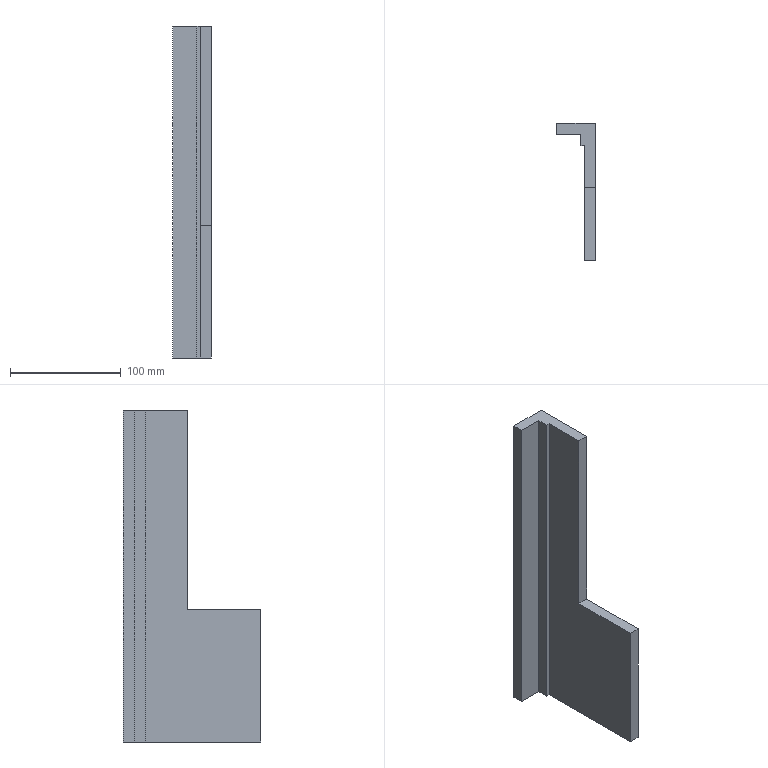Part | STEP file | Platform 2 slider plate 2 | 1 solid | 12 faces | box 35 x 124 x 300 mm | volume 337200 mm3 | plane 12
STEP:
#1=CARTESIAN_POINT('',(0.,0.,-150.));
#2=VERTEX_POINT('',#1);
#3=CARTESIAN_POINT('',(0.,-10.,-150.));
#4=VERTEX_POINT('',#3);
#5=CARTESIAN_POINT('',(0.,-10.,-150.));
#6=DIRECTION('',(0.,-1.,0.));
#7=VECTOR('',#6,1000.);
#8=LINE('',#5,#7);
#9=EDGE_CURVE('',#2,#4,#8,.T.);
#10=ORIENTED_EDGE('',*,*,#9,.T.);
#11=CARTESIAN_POINT('',(0.,-10.,150.));
#12=VERTEX_POINT('',#11);
#13=CARTESIAN_POINT('',(0.,-10.,150.));
#14=DIRECTION('',(0.,0.,-1.));
#15=VECTOR('',#14,1000.);
#16=LINE('',#13,#15);
#17=EDGE_CURVE('',#12,#4,#16,.T.);
#18=ORIENTED_EDGE('',*,*,#17,.F.);
#19=CARTESIAN_POINT('',(0.,0.,150.));
#20=VERTEX_POINT('',#19);
#21=CARTESIAN_POINT('',(0.,-10.,150.));
#22=DIRECTION('',(0.,-1.,0.));
#23=VECTOR('',#22,1000.);
#24=LINE('',#21,#23);
#25=EDGE_CURVE('',#20,#12,#24,.T.);
#26=ORIENTED_EDGE('',*,*,#25,.F.);
#27=CARTESIAN_POINT('',(0.,0.,150.));
#28=DIRECTION('',(0.,0.,-1.));
#29=VECTOR('',#28,1000.);
#30=LINE('',#27,#29);
#31=EDGE_CURVE('',#20,#2,#30,.T.);
#32=ORIENTED_EDGE('',*,*,#31,.T.);
#33=EDGE_LOOP('',(#10,#18,#26,#32));
#34=FACE_OUTER_BOUND('',#33,.T.);
#35=CARTESIAN_POINT('',(0.,-10.,150.));
#36=DIRECTION('',(1.,0.,0.));
#37=DIRECTION('',(0.,0.,-1.));
#38=AXIS2_PLACEMENT_3D('',#35,#36,#37);
#39=PLANE('',#38);
#40=ADVANCED_FACE('',(#34),#39,.F.);
#41=CARTESIAN_POINT('',(22.,-10.,-150.));
#42=VERTEX_POINT('',#41);
#43=CARTESIAN_POINT('',(22.,-10.,-150.));
#44=DIRECTION('',(1.,0.,0.));
#45=VECTOR('',#44,1000.);
#46=LINE('',#43,#45);
#47=EDGE_CURVE('',#4,#42,#46,.T.);
#48=ORIENTED_EDGE('',*,*,#47,.T.);
#49=CARTESIAN_POINT('',(22.,-10.,150.));
#50=VERTEX_POINT('',#49);
#51=CARTESIAN_POINT('',(22.,-10.,150.));
#52=DIRECTION('',(0.,0.,-1.));
#53=VECTOR('',#52,1000.);
#54=LINE('',#51,#53);
#55=EDGE_CURVE('',#50,#42,#54,.T.);
#56=ORIENTED_EDGE('',*,*,#55,.F.);
#57=CARTESIAN_POINT('',(22.,-10.,150.));
#58=DIRECTION('',(1.,0.,0.));
#59=VECTOR('',#58,1000.);
#60=LINE('',#57,#59);
#61=EDGE_CURVE('',#12,#50,#60,.T.);
#62=ORIENTED_EDGE('',*,*,#61,.F.);
#63=ORIENTED_EDGE('',*,*,#17,.T.);
#64=EDGE_LOOP('',(#48,#56,#62,#63));
#65=FACE_OUTER_BOUND('',#64,.T.);
#66=CARTESIAN_POINT('',(22.,-10.,150.));
#67=DIRECTION('',(0.,1.,0.));
#68=DIRECTION('',(-1.,0.,0.));
#69=AXIS2_PLACEMENT_3D('',#66,#67,#68);
#70=PLANE('',#69);
#71=ADVANCED_FACE('',(#65),#70,.F.);
#72=CARTESIAN_POINT('',(22.,-20.,-150.));
#73=VERTEX_POINT('',#72);
#74=CARTESIAN_POINT('',(22.,-124.,-150.));
#75=DIRECTION('',(0.,-1.,0.));
#76=VECTOR('',#75,1000.);
#77=LINE('',#74,#76);
#78=EDGE_CURVE('',#42,#73,#77,.T.);
#79=ORIENTED_EDGE('',*,*,#78,.T.);
#80=CARTESIAN_POINT('',(22.,-20.,150.));
#81=VERTEX_POINT('',#80);
#82=CARTESIAN_POINT('',(22.,-20.,-150.));
#83=DIRECTION('',(0.,0.,1.));
#84=VECTOR('',#83,1000.);
#85=LINE('',#82,#84);
#86=EDGE_CURVE('',#73,#81,#85,.T.);
#87=ORIENTED_EDGE('',*,*,#86,.T.);
#88=CARTESIAN_POINT('',(22.,-124.,150.));
#89=DIRECTION('',(0.,-1.,0.));
#90=VECTOR('',#89,1000.);
#91=LINE('',#88,#90);
#92=EDGE_CURVE('',#50,#81,#91,.T.);
#93=ORIENTED_EDGE('',*,*,#92,.F.);
#94=ORIENTED_EDGE('',*,*,#55,.T.);
#95=EDGE_LOOP('',(#79,#87,#93,#94));
#96=FACE_OUTER_BOUND('',#95,.T.);
#97=CARTESIAN_POINT('',(22.,-124.,150.));
#98=DIRECTION('',(1.,0.,0.));
#99=DIRECTION('',(0.,0.,-1.));
#100=AXIS2_PLACEMENT_3D('',#97,#98,#99);
#101=PLANE('',#100);
#102=ADVANCED_FACE('',(#96),#101,.F.);
#103=CARTESIAN_POINT('',(35.,-124.,-30.));
#104=VERTEX_POINT('',#103);
#105=CARTESIAN_POINT('',(35.,-124.,-150.));
#106=VERTEX_POINT('',#105);
#107=CARTESIAN_POINT('',(35.,-124.,150.));
#108=DIRECTION('',(0.,0.,-1.));
#109=VECTOR('',#108,1000.);
#110=LINE('',#107,#109);
#111=EDGE_CURVE('',#104,#106,#110,.T.);
#112=ORIENTED_EDGE('',*,*,#111,.F.);
#113=CARTESIAN_POINT('',(25.,-124.,-30.));
#114=VERTEX_POINT('',#113);
#115=CARTESIAN_POINT('',(0.,-124.,-30.));
#116=DIRECTION('',(1.,0.,0.));
#117=VECTOR('',#116,1000.);
#118=LINE('',#115,#117);
#119=EDGE_CURVE('',#114,#104,#118,.T.);
#120=ORIENTED_EDGE('',*,*,#119,.F.);
#121=CARTESIAN_POINT('',(25.,-124.,-150.));
#122=VERTEX_POINT('',#121);
#123=CARTESIAN_POINT('',(25.,-124.,-150.));
#124=DIRECTION('',(0.,0.,1.));
#125=VECTOR('',#124,1000.);
#126=LINE('',#123,#125);
#127=EDGE_CURVE('',#122,#114,#126,.T.);
#128=ORIENTED_EDGE('',*,*,#127,.F.);
#129=CARTESIAN_POINT('',(35.,-124.,-150.));
#130=DIRECTION('',(1.,0.,0.));
#131=VECTOR('',#130,1000.);
#132=LINE('',#129,#131);
#133=EDGE_CURVE('',#122,#106,#132,.T.);
#134=ORIENTED_EDGE('',*,*,#133,.T.);
#135=EDGE_LOOP('',(#112,#120,#128,#134));
#136=FACE_OUTER_BOUND('',#135,.T.);
#137=CARTESIAN_POINT('',(35.,-124.,150.));
#138=DIRECTION('',(0.,1.,0.));
#139=DIRECTION('',(0.,0.,1.));
#140=AXIS2_PLACEMENT_3D('',#137,#138,#139);
#141=PLANE('',#140);
#142=ADVANCED_FACE('',(#136),#141,.F.);
#143=CARTESIAN_POINT('',(35.,-58.,150.));
#144=VERTEX_POINT('',#143);
#145=CARTESIAN_POINT('',(35.,0.,150.));
#146=VERTEX_POINT('',#145);
#147=CARTESIAN_POINT('',(35.,0.,150.));
#148=DIRECTION('',(0.,1.,0.));
#149=VECTOR('',#148,1000.);
#150=LINE('',#147,#149);
#151=EDGE_CURVE('',#144,#146,#150,.T.);
#152=ORIENTED_EDGE('',*,*,#151,.F.);
#153=CARTESIAN_POINT('',(35.,-58.,-30.));
#154=VERTEX_POINT('',#153);
#155=CARTESIAN_POINT('',(35.,-58.,150.));
#156=DIRECTION('',(0.,0.,1.));
#157=VECTOR('',#156,1000.);
#158=LINE('',#155,#157);
#159=EDGE_CURVE('',#154,#144,#158,.T.);
#160=ORIENTED_EDGE('',*,*,#159,.F.);
#161=CARTESIAN_POINT('',(35.,-124.,-30.));
#162=DIRECTION('',(0.,1.,0.));
#163=VECTOR('',#162,1000.);
#164=LINE('',#161,#163);
#165=EDGE_CURVE('',#104,#154,#164,.T.);
#166=ORIENTED_EDGE('',*,*,#165,.F.);
#167=ORIENTED_EDGE('',*,*,#111,.T.);
#168=CARTESIAN_POINT('',(35.,0.,-150.));
#169=VERTEX_POINT('',#168);
#170=CARTESIAN_POINT('',(35.,0.,-150.));
#171=DIRECTION('',(0.,1.,0.));
#172=VECTOR('',#171,1000.);
#173=LINE('',#170,#172);
#174=EDGE_CURVE('',#106,#169,#173,.T.);
#175=ORIENTED_EDGE('',*,*,#174,.T.);
#176=CARTESIAN_POINT('',(35.,0.,150.));
#177=DIRECTION('',(0.,0.,-1.));
#178=VECTOR('',#177,1000.);
#179=LINE('',#176,#178);
#180=EDGE_CURVE('',#146,#169,#179,.T.);
#181=ORIENTED_EDGE('',*,*,#180,.F.);
#182=EDGE_LOOP('',(#152,#160,#166,#167,#175,#181));
#183=FACE_OUTER_BOUND('',#182,.T.);
#184=CARTESIAN_POINT('',(35.,0.,150.));
#185=DIRECTION('',(-1.,0.,0.));
#186=DIRECTION('',(0.,-1.,0.));
#187=AXIS2_PLACEMENT_3D('',#184,#185,#186);
#188=PLANE('',#187);
#189=ADVANCED_FACE('',(#183),#188,.F.);
#190=CARTESIAN_POINT('',(0.,0.,-150.));
#191=DIRECTION('',(-1.,0.,0.));
#192=VECTOR('',#191,1000.);
#193=LINE('',#190,#192);
#194=EDGE_CURVE('',#169,#2,#193,.T.);
#195=ORIENTED_EDGE('',*,*,#194,.T.);
#196=ORIENTED_EDGE('',*,*,#31,.F.);
#197=CARTESIAN_POINT('',(0.,0.,150.));
#198=DIRECTION('',(-1.,0.,0.));
#199=VECTOR('',#198,1000.);
#200=LINE('',#197,#199);
#201=EDGE_CURVE('',#146,#20,#200,.T.);
#202=ORIENTED_EDGE('',*,*,#201,.F.);
#203=ORIENTED_EDGE('',*,*,#180,.T.);
#204=EDGE_LOOP('',(#195,#196,#202,#203));
#205=FACE_OUTER_BOUND('',#204,.T.);
#206=CARTESIAN_POINT('',(0.,0.,150.));
#207=DIRECTION('',(0.,-1.,0.));
#208=DIRECTION('',(0.,0.,-1.));
#209=AXIS2_PLACEMENT_3D('',#206,#207,#208);
#210=PLANE('',#209);
#211=ADVANCED_FACE('',(#205),#210,.F.);
#212=CARTESIAN_POINT('',(25.,-58.,150.));
#213=VERTEX_POINT('',#212);
#214=CARTESIAN_POINT('',(25.,-20.,150.));
#215=VERTEX_POINT('',#214);
#216=CARTESIAN_POINT('',(25.,-124.,150.));
#217=DIRECTION('',(0.,1.,0.));
#218=VECTOR('',#217,1000.);
#219=LINE('',#216,#218);
#220=EDGE_CURVE('',#213,#215,#219,.T.);
#221=ORIENTED_EDGE('',*,*,#220,.F.);
#222=CARTESIAN_POINT('',(0.,-58.,150.));
#223=DIRECTION('',(1.,0.,0.));
#224=VECTOR('',#223,1000.);
#225=LINE('',#222,#224);
#226=EDGE_CURVE('',#213,#144,#225,.T.);
#227=ORIENTED_EDGE('',*,*,#226,.T.);
#228=ORIENTED_EDGE('',*,*,#151,.T.);
#229=ORIENTED_EDGE('',*,*,#201,.T.);
#230=ORIENTED_EDGE('',*,*,#25,.T.);
#231=ORIENTED_EDGE('',*,*,#61,.T.);
#232=ORIENTED_EDGE('',*,*,#92,.T.);
#233=CARTESIAN_POINT('',(22.,-20.,150.));
#234=DIRECTION('',(-1.,0.,0.));
#235=VECTOR('',#234,1000.);
#236=LINE('',#233,#235);
#237=EDGE_CURVE('',#215,#81,#236,.T.);
#238=ORIENTED_EDGE('',*,*,#237,.F.);
#239=EDGE_LOOP('',(#221,#227,#228,#229,#230,#231,#232,#238));
#240=FACE_OUTER_BOUND('',#239,.T.);
#241=CARTESIAN_POINT('',(0.,0.,150.));
#242=DIRECTION('',(0.,0.,-1.));
#243=DIRECTION('',(-1.,0.,0.));
#244=AXIS2_PLACEMENT_3D('',#241,#242,#243);
#245=PLANE('',#244);
#246=ADVANCED_FACE('',(#240),#245,.F.);
#247=CARTESIAN_POINT('',(25.,-20.,-150.));
#248=VERTEX_POINT('',#247);
#249=CARTESIAN_POINT('',(22.,-20.,-150.));
#250=DIRECTION('',(-1.,0.,0.));
#251=VECTOR('',#250,1000.);
#252=LINE('',#249,#251);
#253=EDGE_CURVE('',#248,#73,#252,.T.);
#254=ORIENTED_EDGE('',*,*,#253,.T.);
#255=ORIENTED_EDGE('',*,*,#78,.F.);
#256=ORIENTED_EDGE('',*,*,#47,.F.);
#257=ORIENTED_EDGE('',*,*,#9,.F.);
#258=ORIENTED_EDGE('',*,*,#194,.F.);
#259=ORIENTED_EDGE('',*,*,#174,.F.);
#260=ORIENTED_EDGE('',*,*,#133,.F.);
#261=CARTESIAN_POINT('',(25.,-124.,-150.));
#262=DIRECTION('',(0.,1.,0.));
#263=VECTOR('',#262,1000.);
#264=LINE('',#261,#263);
#265=EDGE_CURVE('',#122,#248,#264,.T.);
#266=ORIENTED_EDGE('',*,*,#265,.T.);
#267=EDGE_LOOP('',(#254,#255,#256,#257,#258,#259,#260,#266));
#268=FACE_OUTER_BOUND('',#267,.T.);
#269=CARTESIAN_POINT('',(0.,0.,-150.));
#270=DIRECTION('',(0.,0.,-1.));
#271=DIRECTION('',(-1.,0.,0.));
#272=AXIS2_PLACEMENT_3D('',#269,#270,#271);
#273=PLANE('',#272);
#274=ADVANCED_FACE('',(#268),#273,.T.);
#275=ORIENTED_EDGE('',*,*,#237,.T.);
#276=ORIENTED_EDGE('',*,*,#86,.F.);
#277=ORIENTED_EDGE('',*,*,#253,.F.);
#278=CARTESIAN_POINT('',(25.,-20.,-150.));
#279=DIRECTION('',(0.,0.,1.));
#280=VECTOR('',#279,1000.);
#281=LINE('',#278,#280);
#282=EDGE_CURVE('',#248,#215,#281,.T.);
#283=ORIENTED_EDGE('',*,*,#282,.T.);
#284=EDGE_LOOP('',(#275,#276,#277,#283));
#285=FACE_OUTER_BOUND('',#284,.T.);
#286=CARTESIAN_POINT('',(22.,-20.,-150.));
#287=DIRECTION('',(0.,1.,0.));
#288=DIRECTION('',(0.,0.,1.));
#289=AXIS2_PLACEMENT_3D('',#286,#287,#288);
#290=PLANE('',#289);
#291=ADVANCED_FACE('',(#285),#290,.F.);
#292=CARTESIAN_POINT('',(25.,-58.,-30.));
#293=VERTEX_POINT('',#292);
#294=CARTESIAN_POINT('',(25.,-124.,-30.));
#295=DIRECTION('',(0.,1.,0.));
#296=VECTOR('',#295,1000.);
#297=LINE('',#294,#296);
#298=EDGE_CURVE('',#114,#293,#297,.T.);
#299=ORIENTED_EDGE('',*,*,#298,.T.);
#300=CARTESIAN_POINT('',(25.,-58.,-150.));
#301=DIRECTION('',(0.,0.,1.));
#302=VECTOR('',#301,1000.);
#303=LINE('',#300,#302);
#304=EDGE_CURVE('',#293,#213,#303,.T.);
#305=ORIENTED_EDGE('',*,*,#304,.T.);
#306=ORIENTED_EDGE('',*,*,#220,.T.);
#307=ORIENTED_EDGE('',*,*,#282,.F.);
#308=ORIENTED_EDGE('',*,*,#265,.F.);
#309=ORIENTED_EDGE('',*,*,#127,.T.);
#310=EDGE_LOOP('',(#299,#305,#306,#307,#308,#309));
#311=FACE_OUTER_BOUND('',#310,.T.);
#312=CARTESIAN_POINT('',(25.,-124.,-150.));
#313=DIRECTION('',(1.,0.,0.));
#314=DIRECTION('',(0.,0.,-1.));
#315=AXIS2_PLACEMENT_3D('',#312,#313,#314);
#316=PLANE('',#315);
#317=ADVANCED_FACE('',(#311),#316,.F.);
#318=CARTESIAN_POINT('',(0.,-58.,-30.));
#319=DIRECTION('',(1.,0.,0.));
#320=VECTOR('',#319,1000.);
#321=LINE('',#318,#320);
#322=EDGE_CURVE('',#293,#154,#321,.T.);
#323=ORIENTED_EDGE('',*,*,#322,.T.);
#324=ORIENTED_EDGE('',*,*,#159,.T.);
#325=ORIENTED_EDGE('',*,*,#226,.F.);
#326=ORIENTED_EDGE('',*,*,#304,.F.);
#327=EDGE_LOOP('',(#323,#324,#325,#326));
#328=FACE_OUTER_BOUND('',#327,.T.);
#329=CARTESIAN_POINT('',(0.,-58.,150.));
#330=DIRECTION('',(0.,1.,0.));
#331=DIRECTION('',(-1.,0.,0.));
#332=AXIS2_PLACEMENT_3D('',#329,#330,#331);
#333=PLANE('',#332);
#334=ADVANCED_FACE('',(#328),#333,.F.);
#335=ORIENTED_EDGE('',*,*,#119,.T.);
#336=ORIENTED_EDGE('',*,*,#165,.T.);
#337=ORIENTED_EDGE('',*,*,#322,.F.);
#338=ORIENTED_EDGE('',*,*,#298,.F.);
#339=EDGE_LOOP('',(#335,#336,#337,#338));
#340=FACE_OUTER_BOUND('',#339,.T.);
#341=CARTESIAN_POINT('',(0.,-124.,-30.));
#342=DIRECTION('',(0.,0.,-1.));
#343=DIRECTION('',(-1.,0.,0.));
#344=AXIS2_PLACEMENT_3D('',#341,#342,#343);
#345=PLANE('',#344);
#346=ADVANCED_FACE('',(#340),#345,.F.);
#347=CLOSED_SHELL('',(#40,#71,#102,#142,#189,#211,#246,#274,#291,#317,#334,#346));
#348=MANIFOLD_SOLID_BREP('',#347);
#349=CARTESIAN_POINT('',(0.,0.,0.));
#350=DIRECTION('',(0.,0.,1.));
#351=DIRECTION('',(1.,0.,0.));
#352=AXIS2_PLACEMENT_3D('',#349,#350,#351);
#353=(LENGTH_UNIT()NAMED_UNIT(*)SI_UNIT(.MILLI.,.METRE.));
#354=UNCERTAINTY_MEASURE_WITH_UNIT(LENGTH_MEASURE(0.00001),#353,'','');
#355=(NAMED_UNIT(*)PLANE_ANGLE_UNIT()SI_UNIT($,.RADIAN.));
#356=(NAMED_UNIT(*)SI_UNIT($,.STERADIAN.)SOLID_ANGLE_UNIT());
#357=(GEOMETRIC_REPRESENTATION_CONTEXT(3)GLOBAL_UNCERTAINTY_ASSIGNED_CONTEXT((#354))GLOBAL_UNIT_ASSIGNED_CONTEXT((#353,#355,#356))REPRESENTATION_CONTEXT('',''));
#358=ADVANCED_BREP_SHAPE_REPRESENTATION('',(#348,#352),#357);